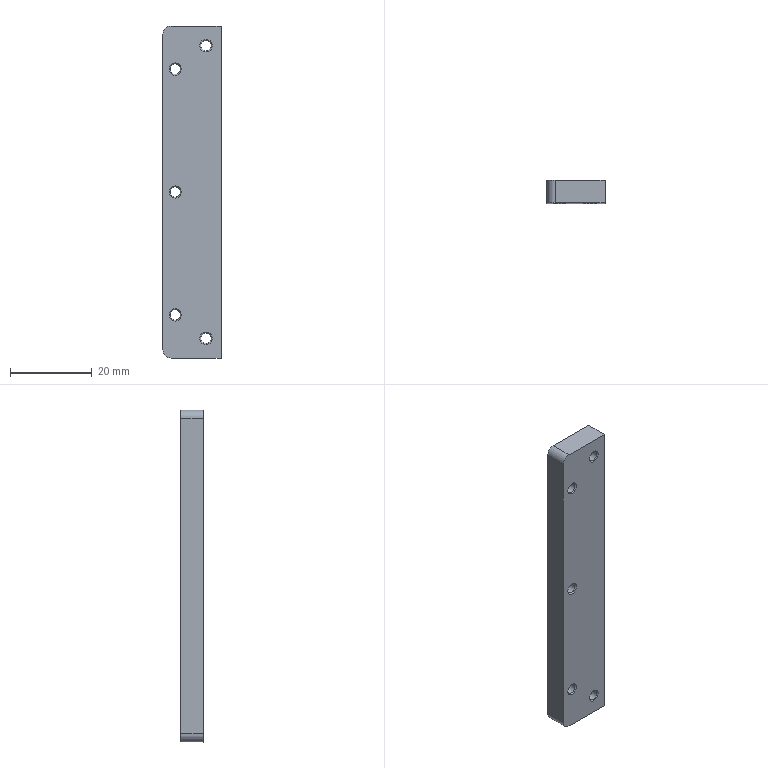Part | STEP file | Screen mounting block 2 | 1 solid | 23 faces | box 14.19 x 5.5 x 81 mm | volume 6175 mm3 | cone 10 | cylinder 7 | plane 6 | commonest cylinder face diameters 2.5 x5 4 x2